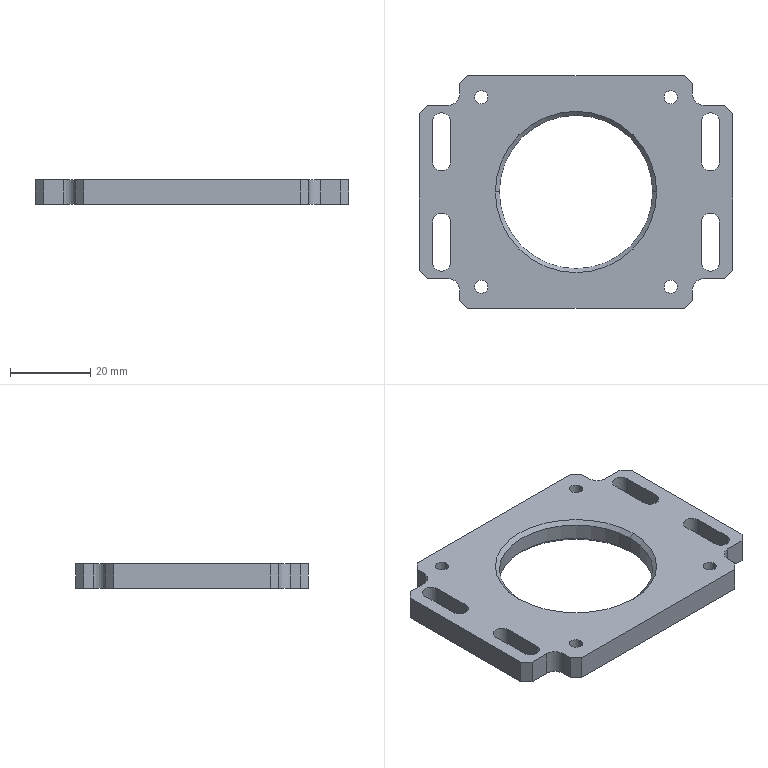Part | NX | features BREP 1 | 1 solid | 56 faces | box 78 x 58 x 6 mm | volume 16629 mm3 | plane 30 | cylinder 22 | cone 4 | commonest cylinder face diameters 3.3 x8 4.5 x8 6 x4 38.2 x2